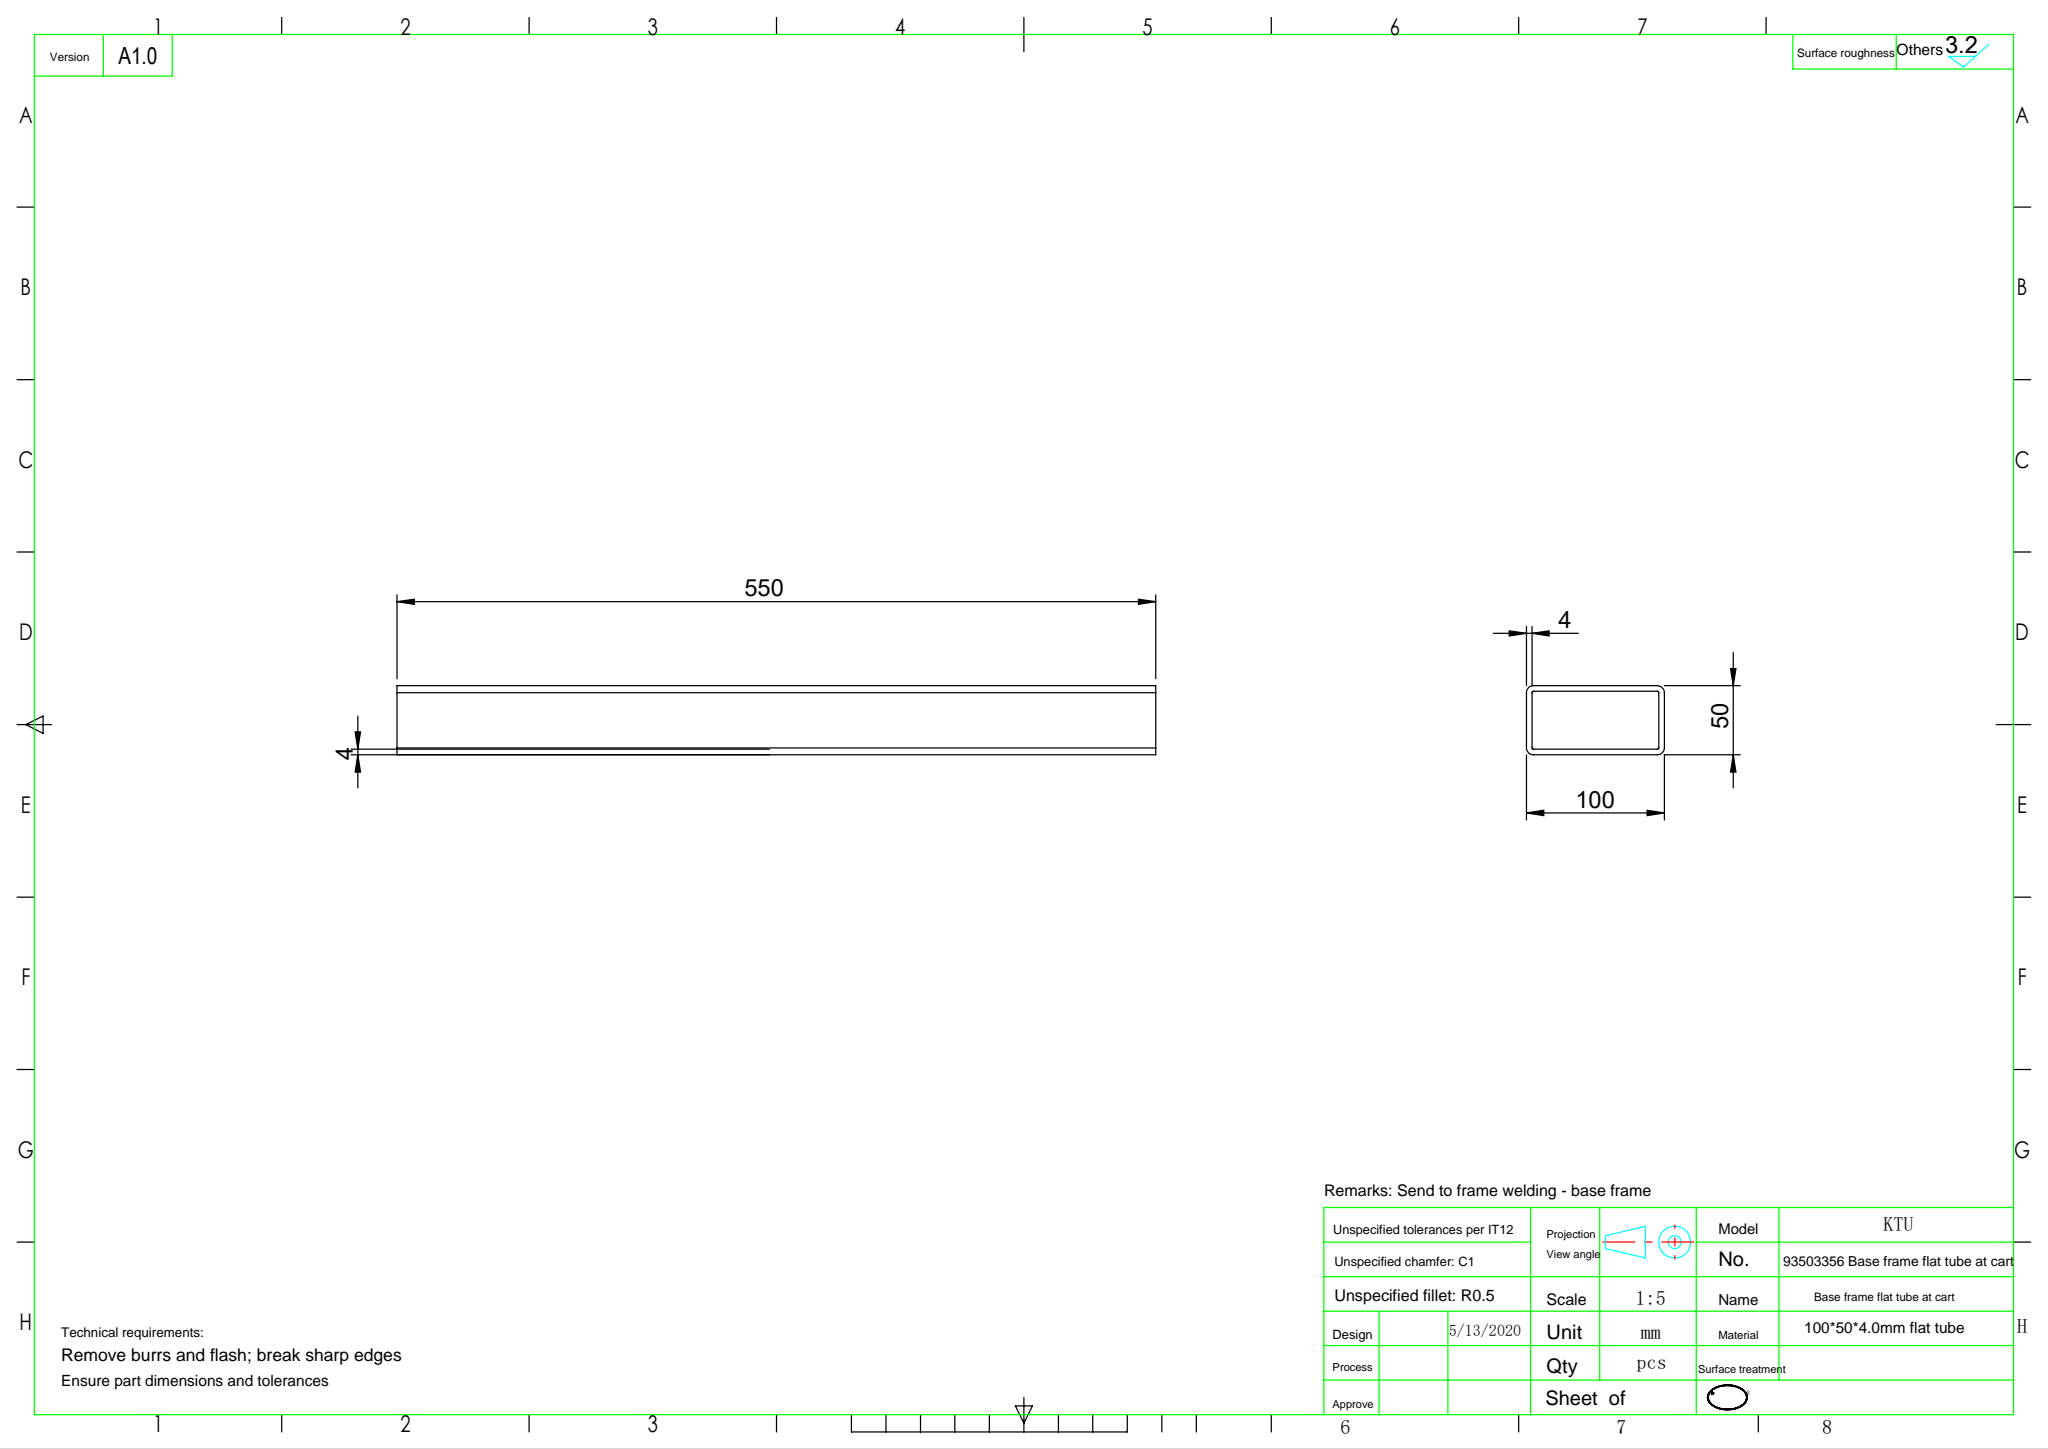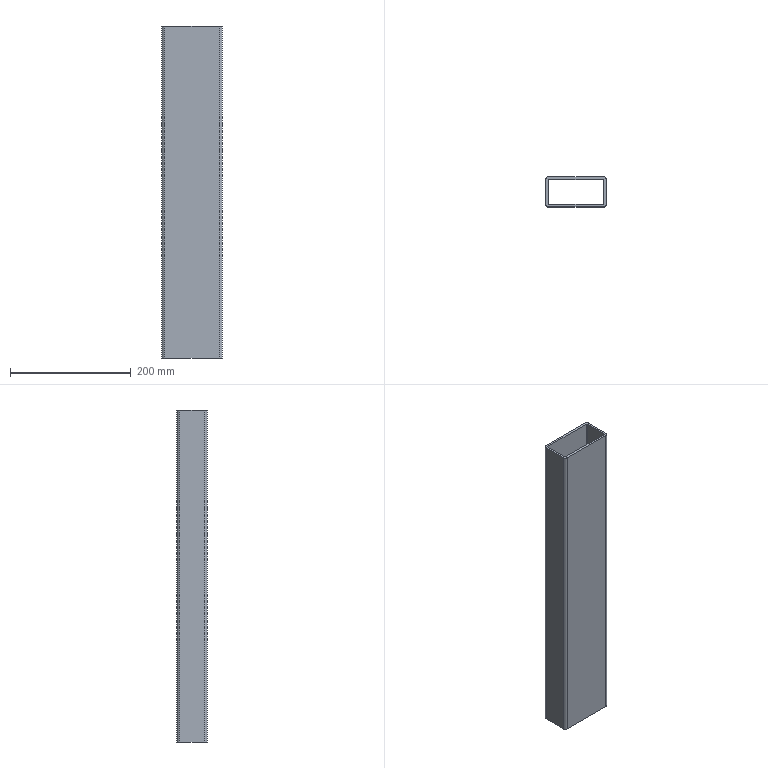Part | SolidWorks | features ExtruThin 1 | 1 solid | 18 faces | box 100 x 50 x 550 mm | volume 613469 mm3 | plane 10 | cylinder 8 | commonest cylinder face diameters 2 x4 10 x4
STEP:
#1=CARTESIAN_POINT('',(45.,-25.,275.));
#2=VERTEX_POINT('',#1);
#3=CARTESIAN_POINT('',(50.,-20.,275.));
#4=VERTEX_POINT('',#3);
#5=CARTESIAN_POINT('',(45.,-20.,275.));
#6=DIRECTION('',(0.,0.,1.));
#7=DIRECTION('',(1.,0.,0.));
#8=AXIS2_PLACEMENT_3D('',#5,#6,#7);
#9=CIRCLE('',#8,5.);
#10=EDGE_CURVE('',#2,#4,#9,.T.);
#11=ORIENTED_EDGE('',*,*,#10,.T.);
#12=CARTESIAN_POINT('',(50.,20.,275.));
#13=VERTEX_POINT('',#12);
#14=CARTESIAN_POINT('',(50.,20.,275.));
#15=DIRECTION('',(0.,1.,0.));
#16=VECTOR('',#15,1000.);
#17=LINE('',#14,#16);
#18=EDGE_CURVE('',#4,#13,#17,.T.);
#19=ORIENTED_EDGE('',*,*,#18,.T.);
#20=CARTESIAN_POINT('',(45.,25.,275.));
#21=VERTEX_POINT('',#20);
#22=CARTESIAN_POINT('',(45.,20.,275.));
#23=DIRECTION('',(0.,0.,1.));
#24=DIRECTION('',(-1.,0.,0.));
#25=AXIS2_PLACEMENT_3D('',#22,#23,#24);
#26=CIRCLE('',#25,5.);
#27=EDGE_CURVE('',#13,#21,#26,.T.);
#28=ORIENTED_EDGE('',*,*,#27,.T.);
#29=CARTESIAN_POINT('',(-45.,25.,275.));
#30=VERTEX_POINT('',#29);
#31=CARTESIAN_POINT('',(-45.,25.,275.));
#32=DIRECTION('',(-1.,0.,0.));
#33=VECTOR('',#32,1000.);
#34=LINE('',#31,#33);
#35=EDGE_CURVE('',#21,#30,#34,.T.);
#36=ORIENTED_EDGE('',*,*,#35,.T.);
#37=CARTESIAN_POINT('',(-50.,20.,275.));
#38=VERTEX_POINT('',#37);
#39=CARTESIAN_POINT('',(-45.,20.,275.));
#40=DIRECTION('',(0.,0.,1.));
#41=DIRECTION('',(1.,0.,0.));
#42=AXIS2_PLACEMENT_3D('',#39,#40,#41);
#43=CIRCLE('',#42,5.);
#44=EDGE_CURVE('',#30,#38,#43,.T.);
#45=ORIENTED_EDGE('',*,*,#44,.T.);
#46=CARTESIAN_POINT('',(-50.,-20.,275.));
#47=VERTEX_POINT('',#46);
#48=CARTESIAN_POINT('',(-50.,20.,275.));
#49=DIRECTION('',(0.,-1.,0.));
#50=VECTOR('',#49,1000.);
#51=LINE('',#48,#50);
#52=EDGE_CURVE('',#38,#47,#51,.T.);
#53=ORIENTED_EDGE('',*,*,#52,.T.);
#54=CARTESIAN_POINT('',(-45.,-25.,275.));
#55=VERTEX_POINT('',#54);
#56=CARTESIAN_POINT('',(-45.,-20.,275.));
#57=DIRECTION('',(0.,0.,1.));
#58=DIRECTION('',(1.,0.,0.));
#59=AXIS2_PLACEMENT_3D('',#56,#57,#58);
#60=CIRCLE('',#59,5.);
#61=EDGE_CURVE('',#47,#55,#60,.T.);
#62=ORIENTED_EDGE('',*,*,#61,.T.);
#63=CARTESIAN_POINT('',(-45.,-25.,275.));
#64=DIRECTION('',(1.,0.,0.));
#65=VECTOR('',#64,1000.);
#66=LINE('',#63,#65);
#67=EDGE_CURVE('',#55,#2,#66,.T.);
#68=ORIENTED_EDGE('',*,*,#67,.T.);
#69=EDGE_LOOP('',(#11,#19,#28,#36,#45,#53,#62,#68));
#70=FACE_OUTER_BOUND('',#69,.T.);
#71=CARTESIAN_POINT('',(46.,-20.,275.));
#72=VERTEX_POINT('',#71);
#73=CARTESIAN_POINT('',(46.,20.,275.));
#74=VERTEX_POINT('',#73);
#75=CARTESIAN_POINT('',(46.,20.,275.));
#76=DIRECTION('',(0.,1.,0.));
#77=VECTOR('',#76,1000.);
#78=LINE('',#75,#77);
#79=EDGE_CURVE('',#72,#74,#78,.T.);
#80=ORIENTED_EDGE('',*,*,#79,.F.);
#81=CARTESIAN_POINT('',(45.,-21.,275.));
#82=VERTEX_POINT('',#81);
#83=CARTESIAN_POINT('',(45.,-20.,275.));
#84=DIRECTION('',(0.,0.,1.));
#85=DIRECTION('',(1.,0.,0.));
#86=AXIS2_PLACEMENT_3D('',#83,#84,#85);
#87=CIRCLE('',#86,1.);
#88=EDGE_CURVE('',#82,#72,#87,.T.);
#89=ORIENTED_EDGE('',*,*,#88,.F.);
#90=CARTESIAN_POINT('',(-45.,-21.,275.));
#91=VERTEX_POINT('',#90);
#92=CARTESIAN_POINT('',(-45.,-21.,275.));
#93=DIRECTION('',(1.,0.,0.));
#94=VECTOR('',#93,1000.);
#95=LINE('',#92,#94);
#96=EDGE_CURVE('',#91,#82,#95,.T.);
#97=ORIENTED_EDGE('',*,*,#96,.F.);
#98=CARTESIAN_POINT('',(-46.,-20.,275.));
#99=VERTEX_POINT('',#98);
#100=CARTESIAN_POINT('',(-45.,-20.,275.));
#101=DIRECTION('',(0.,0.,1.));
#102=DIRECTION('',(1.,0.,0.));
#103=AXIS2_PLACEMENT_3D('',#100,#101,#102);
#104=CIRCLE('',#103,1.);
#105=EDGE_CURVE('',#99,#91,#104,.T.);
#106=ORIENTED_EDGE('',*,*,#105,.F.);
#107=CARTESIAN_POINT('',(-46.,20.,275.));
#108=VERTEX_POINT('',#107);
#109=CARTESIAN_POINT('',(-46.,20.,275.));
#110=DIRECTION('',(0.,-1.,0.));
#111=VECTOR('',#110,1000.);
#112=LINE('',#109,#111);
#113=EDGE_CURVE('',#108,#99,#112,.T.);
#114=ORIENTED_EDGE('',*,*,#113,.F.);
#115=CARTESIAN_POINT('',(-45.,21.,275.));
#116=VERTEX_POINT('',#115);
#117=CARTESIAN_POINT('',(-45.,20.,275.));
#118=DIRECTION('',(0.,0.,1.));
#119=DIRECTION('',(1.,0.,0.));
#120=AXIS2_PLACEMENT_3D('',#117,#118,#119);
#121=CIRCLE('',#120,1.);
#122=EDGE_CURVE('',#116,#108,#121,.T.);
#123=ORIENTED_EDGE('',*,*,#122,.F.);
#124=CARTESIAN_POINT('',(45.,21.,275.));
#125=VERTEX_POINT('',#124);
#126=CARTESIAN_POINT('',(-45.,21.,275.));
#127=DIRECTION('',(-1.,0.,0.));
#128=VECTOR('',#127,1000.);
#129=LINE('',#126,#128);
#130=EDGE_CURVE('',#125,#116,#129,.T.);
#131=ORIENTED_EDGE('',*,*,#130,.F.);
#132=CARTESIAN_POINT('',(45.,20.,275.));
#133=DIRECTION('',(0.,0.,1.));
#134=DIRECTION('',(1.,0.,0.));
#135=AXIS2_PLACEMENT_3D('',#132,#133,#134);
#136=CIRCLE('',#135,1.);
#137=EDGE_CURVE('',#74,#125,#136,.T.);
#138=ORIENTED_EDGE('',*,*,#137,.F.);
#139=EDGE_LOOP('',(#80,#89,#97,#106,#114,#123,#131,#138));
#140=FACE_BOUND('',#139,.T.);
#141=CARTESIAN_POINT('',(45.,-20.,275.));
#142=DIRECTION('',(0.,0.,1.));
#143=DIRECTION('',(1.,0.,0.));
#144=AXIS2_PLACEMENT_3D('',#141,#142,#143);
#145=PLANE('',#144);
#146=ADVANCED_FACE('',(#70,#140),#145,.T.);
#147=CARTESIAN_POINT('',(45.,-25.,-275.));
#148=VERTEX_POINT('',#147);
#149=CARTESIAN_POINT('',(50.,-20.,-275.));
#150=VERTEX_POINT('',#149);
#151=CARTESIAN_POINT('',(45.,-20.,-275.));
#152=DIRECTION('',(0.,0.,1.));
#153=DIRECTION('',(1.,0.,0.));
#154=AXIS2_PLACEMENT_3D('',#151,#152,#153);
#155=CIRCLE('',#154,5.);
#156=EDGE_CURVE('',#148,#150,#155,.T.);
#157=ORIENTED_EDGE('',*,*,#156,.F.);
#158=CARTESIAN_POINT('',(-45.,-25.,-275.));
#159=VERTEX_POINT('',#158);
#160=CARTESIAN_POINT('',(-45.,-25.,-275.));
#161=DIRECTION('',(1.,0.,0.));
#162=VECTOR('',#161,1000.);
#163=LINE('',#160,#162);
#164=EDGE_CURVE('',#159,#148,#163,.T.);
#165=ORIENTED_EDGE('',*,*,#164,.F.);
#166=CARTESIAN_POINT('',(-50.,-20.,-275.));
#167=VERTEX_POINT('',#166);
#168=CARTESIAN_POINT('',(-45.,-20.,-275.));
#169=DIRECTION('',(0.,0.,1.));
#170=DIRECTION('',(1.,0.,0.));
#171=AXIS2_PLACEMENT_3D('',#168,#169,#170);
#172=CIRCLE('',#171,5.);
#173=EDGE_CURVE('',#167,#159,#172,.T.);
#174=ORIENTED_EDGE('',*,*,#173,.F.);
#175=CARTESIAN_POINT('',(-50.,20.,-275.));
#176=VERTEX_POINT('',#175);
#177=CARTESIAN_POINT('',(-50.,20.,-275.));
#178=DIRECTION('',(0.,-1.,0.));
#179=VECTOR('',#178,1000.);
#180=LINE('',#177,#179);
#181=EDGE_CURVE('',#176,#167,#180,.T.);
#182=ORIENTED_EDGE('',*,*,#181,.F.);
#183=CARTESIAN_POINT('',(-45.,25.,-275.));
#184=VERTEX_POINT('',#183);
#185=CARTESIAN_POINT('',(-45.,20.,-275.));
#186=DIRECTION('',(0.,0.,1.));
#187=DIRECTION('',(1.,0.,0.));
#188=AXIS2_PLACEMENT_3D('',#185,#186,#187);
#189=CIRCLE('',#188,5.);
#190=EDGE_CURVE('',#184,#176,#189,.T.);
#191=ORIENTED_EDGE('',*,*,#190,.F.);
#192=CARTESIAN_POINT('',(45.,25.,-275.));
#193=VERTEX_POINT('',#192);
#194=CARTESIAN_POINT('',(-45.,25.,-275.));
#195=DIRECTION('',(-1.,0.,0.));
#196=VECTOR('',#195,1000.);
#197=LINE('',#194,#196);
#198=EDGE_CURVE('',#193,#184,#197,.T.);
#199=ORIENTED_EDGE('',*,*,#198,.F.);
#200=CARTESIAN_POINT('',(50.,20.,-275.));
#201=VERTEX_POINT('',#200);
#202=CARTESIAN_POINT('',(45.,20.,-275.));
#203=DIRECTION('',(0.,0.,1.));
#204=DIRECTION('',(-1.,0.,0.));
#205=AXIS2_PLACEMENT_3D('',#202,#203,#204);
#206=CIRCLE('',#205,5.);
#207=EDGE_CURVE('',#201,#193,#206,.T.);
#208=ORIENTED_EDGE('',*,*,#207,.F.);
#209=CARTESIAN_POINT('',(50.,20.,-275.));
#210=DIRECTION('',(0.,1.,0.));
#211=VECTOR('',#210,1000.);
#212=LINE('',#209,#211);
#213=EDGE_CURVE('',#150,#201,#212,.T.);
#214=ORIENTED_EDGE('',*,*,#213,.F.);
#215=EDGE_LOOP('',(#157,#165,#174,#182,#191,#199,#208,#214));
#216=FACE_OUTER_BOUND('',#215,.T.);
#217=CARTESIAN_POINT('',(45.,-21.,-275.));
#218=VERTEX_POINT('',#217);
#219=CARTESIAN_POINT('',(46.,-20.,-275.));
#220=VERTEX_POINT('',#219);
#221=CARTESIAN_POINT('',(45.,-20.,-275.));
#222=DIRECTION('',(0.,0.,1.));
#223=DIRECTION('',(1.,0.,0.));
#224=AXIS2_PLACEMENT_3D('',#221,#222,#223);
#225=CIRCLE('',#224,1.);
#226=EDGE_CURVE('',#218,#220,#225,.T.);
#227=ORIENTED_EDGE('',*,*,#226,.T.);
#228=CARTESIAN_POINT('',(46.,20.,-275.));
#229=VERTEX_POINT('',#228);
#230=CARTESIAN_POINT('',(46.,20.,-275.));
#231=DIRECTION('',(0.,1.,0.));
#232=VECTOR('',#231,1000.);
#233=LINE('',#230,#232);
#234=EDGE_CURVE('',#220,#229,#233,.T.);
#235=ORIENTED_EDGE('',*,*,#234,.T.);
#236=CARTESIAN_POINT('',(45.,21.,-275.));
#237=VERTEX_POINT('',#236);
#238=CARTESIAN_POINT('',(45.,20.,-275.));
#239=DIRECTION('',(0.,0.,1.));
#240=DIRECTION('',(1.,0.,0.));
#241=AXIS2_PLACEMENT_3D('',#238,#239,#240);
#242=CIRCLE('',#241,1.);
#243=EDGE_CURVE('',#229,#237,#242,.T.);
#244=ORIENTED_EDGE('',*,*,#243,.T.);
#245=CARTESIAN_POINT('',(-45.,21.,-275.));
#246=VERTEX_POINT('',#245);
#247=CARTESIAN_POINT('',(-45.,21.,-275.));
#248=DIRECTION('',(-1.,0.,0.));
#249=VECTOR('',#248,1000.);
#250=LINE('',#247,#249);
#251=EDGE_CURVE('',#237,#246,#250,.T.);
#252=ORIENTED_EDGE('',*,*,#251,.T.);
#253=CARTESIAN_POINT('',(-46.,20.,-275.));
#254=VERTEX_POINT('',#253);
#255=CARTESIAN_POINT('',(-45.,20.,-275.));
#256=DIRECTION('',(0.,0.,1.));
#257=DIRECTION('',(1.,0.,0.));
#258=AXIS2_PLACEMENT_3D('',#255,#256,#257);
#259=CIRCLE('',#258,1.);
#260=EDGE_CURVE('',#246,#254,#259,.T.);
#261=ORIENTED_EDGE('',*,*,#260,.T.);
#262=CARTESIAN_POINT('',(-46.,-20.,-275.));
#263=VERTEX_POINT('',#262);
#264=CARTESIAN_POINT('',(-46.,20.,-275.));
#265=DIRECTION('',(0.,-1.,0.));
#266=VECTOR('',#265,1000.);
#267=LINE('',#264,#266);
#268=EDGE_CURVE('',#254,#263,#267,.T.);
#269=ORIENTED_EDGE('',*,*,#268,.T.);
#270=CARTESIAN_POINT('',(-45.,-21.,-275.));
#271=VERTEX_POINT('',#270);
#272=CARTESIAN_POINT('',(-45.,-20.,-275.));
#273=DIRECTION('',(0.,0.,1.));
#274=DIRECTION('',(1.,0.,0.));
#275=AXIS2_PLACEMENT_3D('',#272,#273,#274);
#276=CIRCLE('',#275,1.);
#277=EDGE_CURVE('',#263,#271,#276,.T.);
#278=ORIENTED_EDGE('',*,*,#277,.T.);
#279=CARTESIAN_POINT('',(-45.,-21.,-275.));
#280=DIRECTION('',(1.,0.,0.));
#281=VECTOR('',#280,1000.);
#282=LINE('',#279,#281);
#283=EDGE_CURVE('',#271,#218,#282,.T.);
#284=ORIENTED_EDGE('',*,*,#283,.T.);
#285=EDGE_LOOP('',(#227,#235,#244,#252,#261,#269,#278,#284));
#286=FACE_BOUND('',#285,.T.);
#287=CARTESIAN_POINT('',(45.,-20.,-275.));
#288=DIRECTION('',(0.,0.,1.));
#289=DIRECTION('',(1.,0.,0.));
#290=AXIS2_PLACEMENT_3D('',#287,#288,#289);
#291=PLANE('',#290);
#292=ADVANCED_FACE('',(#216,#286),#291,.F.);
#293=ORIENTED_EDGE('',*,*,#156,.T.);
#294=CARTESIAN_POINT('',(50.,-20.,275.));
#295=DIRECTION('',(0.,0.,-1.));
#296=VECTOR('',#295,1000.);
#297=LINE('',#294,#296);
#298=EDGE_CURVE('',#4,#150,#297,.T.);
#299=ORIENTED_EDGE('',*,*,#298,.F.);
#300=ORIENTED_EDGE('',*,*,#10,.F.);
#301=CARTESIAN_POINT('',(45.,-25.,275.));
#302=DIRECTION('',(0.,0.,-1.));
#303=VECTOR('',#302,1000.);
#304=LINE('',#301,#303);
#305=EDGE_CURVE('',#2,#148,#304,.T.);
#306=ORIENTED_EDGE('',*,*,#305,.T.);
#307=EDGE_LOOP('',(#293,#299,#300,#306));
#308=FACE_OUTER_BOUND('',#307,.T.);
#309=CARTESIAN_POINT('',(45.,-20.,275.));
#310=DIRECTION('',(0.,0.,-1.));
#311=DIRECTION('',(-1.,0.,0.));
#312=AXIS2_PLACEMENT_3D('',#309,#310,#311);
#313=CYLINDRICAL_SURFACE('',#312,5.);
#314=ADVANCED_FACE('',(#308),#313,.T.);
#315=ORIENTED_EDGE('',*,*,#213,.T.);
#316=CARTESIAN_POINT('',(50.,20.,275.));
#317=DIRECTION('',(0.,0.,-1.));
#318=VECTOR('',#317,1000.);
#319=LINE('',#316,#318);
#320=EDGE_CURVE('',#13,#201,#319,.T.);
#321=ORIENTED_EDGE('',*,*,#320,.F.);
#322=ORIENTED_EDGE('',*,*,#18,.F.);
#323=ORIENTED_EDGE('',*,*,#298,.T.);
#324=EDGE_LOOP('',(#315,#321,#322,#323));
#325=FACE_OUTER_BOUND('',#324,.T.);
#326=CARTESIAN_POINT('',(50.,20.,275.));
#327=DIRECTION('',(-1.,0.,0.));
#328=DIRECTION('',(0.,-1.,0.));
#329=AXIS2_PLACEMENT_3D('',#326,#327,#328);
#330=PLANE('',#329);
#331=ADVANCED_FACE('',(#325),#330,.F.);
#332=ORIENTED_EDGE('',*,*,#207,.T.);
#333=CARTESIAN_POINT('',(45.,25.,275.));
#334=DIRECTION('',(0.,0.,-1.));
#335=VECTOR('',#334,1000.);
#336=LINE('',#333,#335);
#337=EDGE_CURVE('',#21,#193,#336,.T.);
#338=ORIENTED_EDGE('',*,*,#337,.F.);
#339=ORIENTED_EDGE('',*,*,#27,.F.);
#340=ORIENTED_EDGE('',*,*,#320,.T.);
#341=EDGE_LOOP('',(#332,#338,#339,#340));
#342=FACE_OUTER_BOUND('',#341,.T.);
#343=CARTESIAN_POINT('',(45.,20.,275.));
#344=DIRECTION('',(0.,0.,-1.));
#345=DIRECTION('',(-1.,0.,0.));
#346=AXIS2_PLACEMENT_3D('',#343,#344,#345);
#347=CYLINDRICAL_SURFACE('',#346,5.);
#348=ADVANCED_FACE('',(#342),#347,.T.);
#349=ORIENTED_EDGE('',*,*,#198,.T.);
#350=CARTESIAN_POINT('',(-45.,25.,275.));
#351=DIRECTION('',(0.,0.,-1.));
#352=VECTOR('',#351,1000.);
#353=LINE('',#350,#352);
#354=EDGE_CURVE('',#30,#184,#353,.T.);
#355=ORIENTED_EDGE('',*,*,#354,.F.);
#356=ORIENTED_EDGE('',*,*,#35,.F.);
#357=ORIENTED_EDGE('',*,*,#337,.T.);
#358=EDGE_LOOP('',(#349,#355,#356,#357));
#359=FACE_OUTER_BOUND('',#358,.T.);
#360=CARTESIAN_POINT('',(-45.,25.,275.));
#361=DIRECTION('',(0.,-1.,0.));
#362=DIRECTION('',(0.,0.,-1.));
#363=AXIS2_PLACEMENT_3D('',#360,#361,#362);
#364=PLANE('',#363);
#365=ADVANCED_FACE('',(#359),#364,.F.);
#366=ORIENTED_EDGE('',*,*,#190,.T.);
#367=CARTESIAN_POINT('',(-50.,20.,275.));
#368=DIRECTION('',(0.,0.,-1.));
#369=VECTOR('',#368,1000.);
#370=LINE('',#367,#369);
#371=EDGE_CURVE('',#38,#176,#370,.T.);
#372=ORIENTED_EDGE('',*,*,#371,.F.);
#373=ORIENTED_EDGE('',*,*,#44,.F.);
#374=ORIENTED_EDGE('',*,*,#354,.T.);
#375=EDGE_LOOP('',(#366,#372,#373,#374));
#376=FACE_OUTER_BOUND('',#375,.T.);
#377=CARTESIAN_POINT('',(-45.,20.,275.));
#378=DIRECTION('',(0.,0.,-1.));
#379=DIRECTION('',(-1.,0.,0.));
#380=AXIS2_PLACEMENT_3D('',#377,#378,#379);
#381=CYLINDRICAL_SURFACE('',#380,5.);
#382=ADVANCED_FACE('',(#376),#381,.T.);
#383=ORIENTED_EDGE('',*,*,#181,.T.);
#384=CARTESIAN_POINT('',(-50.,-20.,275.));
#385=DIRECTION('',(0.,0.,-1.));
#386=VECTOR('',#385,1000.);
#387=LINE('',#384,#386);
#388=EDGE_CURVE('',#47,#167,#387,.T.);
#389=ORIENTED_EDGE('',*,*,#388,.F.);
#390=ORIENTED_EDGE('',*,*,#52,.F.);
#391=ORIENTED_EDGE('',*,*,#371,.T.);
#392=EDGE_LOOP('',(#383,#389,#390,#391));
#393=FACE_OUTER_BOUND('',#392,.T.);
#394=CARTESIAN_POINT('',(-50.,20.,275.));
#395=DIRECTION('',(1.,0.,0.));
#396=DIRECTION('',(0.,0.,-1.));
#397=AXIS2_PLACEMENT_3D('',#394,#395,#396);
#398=PLANE('',#397);
#399=ADVANCED_FACE('',(#393),#398,.F.);
#400=ORIENTED_EDGE('',*,*,#173,.T.);
#401=CARTESIAN_POINT('',(-45.,-25.,275.));
#402=DIRECTION('',(0.,0.,-1.));
#403=VECTOR('',#402,1000.);
#404=LINE('',#401,#403);
#405=EDGE_CURVE('',#55,#159,#404,.T.);
#406=ORIENTED_EDGE('',*,*,#405,.F.);
#407=ORIENTED_EDGE('',*,*,#61,.F.);
#408=ORIENTED_EDGE('',*,*,#388,.T.);
#409=EDGE_LOOP('',(#400,#406,#407,#408));
#410=FACE_OUTER_BOUND('',#409,.T.);
#411=CARTESIAN_POINT('',(-45.,-20.,275.));
#412=DIRECTION('',(0.,0.,-1.));
#413=DIRECTION('',(-1.,0.,0.));
#414=AXIS2_PLACEMENT_3D('',#411,#412,#413);
#415=CYLINDRICAL_SURFACE('',#414,5.);
#416=ADVANCED_FACE('',(#410),#415,.T.);
#417=ORIENTED_EDGE('',*,*,#164,.T.);
#418=ORIENTED_EDGE('',*,*,#305,.F.);
#419=ORIENTED_EDGE('',*,*,#67,.F.);
#420=ORIENTED_EDGE('',*,*,#405,.T.);
#421=EDGE_LOOP('',(#417,#418,#419,#420));
#422=FACE_OUTER_BOUND('',#421,.T.);
#423=CARTESIAN_POINT('',(-45.,-25.,275.));
#424=DIRECTION('',(0.,1.,0.));
#425=DIRECTION('',(0.,0.,1.));
#426=AXIS2_PLACEMENT_3D('',#423,#424,#425);
#427=PLANE('',#426);
#428=ADVANCED_FACE('',(#422),#427,.F.);
#429=ORIENTED_EDGE('',*,*,#226,.F.);
#430=CARTESIAN_POINT('',(45.,-21.,275.));
#431=DIRECTION('',(0.,0.,-1.));
#432=VECTOR('',#431,1000.);
#433=LINE('',#430,#432);
#434=EDGE_CURVE('',#82,#218,#433,.T.);
#435=ORIENTED_EDGE('',*,*,#434,.F.);
#436=ORIENTED_EDGE('',*,*,#88,.T.);
#437=CARTESIAN_POINT('',(46.,-20.,275.));
#438=DIRECTION('',(0.,0.,-1.));
#439=VECTOR('',#438,1000.);
#440=LINE('',#437,#439);
#441=EDGE_CURVE('',#72,#220,#440,.T.);
#442=ORIENTED_EDGE('',*,*,#441,.T.);
#443=EDGE_LOOP('',(#429,#435,#436,#442));
#444=FACE_OUTER_BOUND('',#443,.T.);
#445=CARTESIAN_POINT('',(45.,-20.,275.));
#446=DIRECTION('',(0.,0.,-1.));
#447=DIRECTION('',(-1.,0.,0.));
#448=AXIS2_PLACEMENT_3D('',#445,#446,#447);
#449=CYLINDRICAL_SURFACE('',#448,1.);
#450=ADVANCED_FACE('',(#444),#449,.F.);
#451=ORIENTED_EDGE('',*,*,#234,.F.);
#452=ORIENTED_EDGE('',*,*,#441,.F.);
#453=ORIENTED_EDGE('',*,*,#79,.T.);
#454=CARTESIAN_POINT('',(46.,20.,275.));
#455=DIRECTION('',(0.,0.,-1.));
#456=VECTOR('',#455,1000.);
#457=LINE('',#454,#456);
#458=EDGE_CURVE('',#74,#229,#457,.T.);
#459=ORIENTED_EDGE('',*,*,#458,.T.);
#460=EDGE_LOOP('',(#451,#452,#453,#459));
#461=FACE_OUTER_BOUND('',#460,.T.);
#462=CARTESIAN_POINT('',(46.,20.,275.));
#463=DIRECTION('',(-1.,0.,0.));
#464=DIRECTION('',(0.,-1.,0.));
#465=AXIS2_PLACEMENT_3D('',#462,#463,#464);
#466=PLANE('',#465);
#467=ADVANCED_FACE('',(#461),#466,.T.);
#468=ORIENTED_EDGE('',*,*,#243,.F.);
#469=ORIENTED_EDGE('',*,*,#458,.F.);
#470=ORIENTED_EDGE('',*,*,#137,.T.);
#471=CARTESIAN_POINT('',(45.,21.,275.));
#472=DIRECTION('',(0.,0.,-1.));
#473=VECTOR('',#472,1000.);
#474=LINE('',#471,#473);
#475=EDGE_CURVE('',#125,#237,#474,.T.);
#476=ORIENTED_EDGE('',*,*,#475,.T.);
#477=EDGE_LOOP('',(#468,#469,#470,#476));
#478=FACE_OUTER_BOUND('',#477,.T.);
#479=CARTESIAN_POINT('',(45.,20.,275.));
#480=DIRECTION('',(0.,0.,-1.));
#481=DIRECTION('',(-1.,0.,0.));
#482=AXIS2_PLACEMENT_3D('',#479,#480,#481);
#483=CYLINDRICAL_SURFACE('',#482,1.);
#484=ADVANCED_FACE('',(#478),#483,.F.);
#485=ORIENTED_EDGE('',*,*,#251,.F.);
#486=ORIENTED_EDGE('',*,*,#475,.F.);
#487=ORIENTED_EDGE('',*,*,#130,.T.);
#488=CARTESIAN_POINT('',(-45.,21.,275.));
#489=DIRECTION('',(0.,0.,-1.));
#490=VECTOR('',#489,1000.);
#491=LINE('',#488,#490);
#492=EDGE_CURVE('',#116,#246,#491,.T.);
#493=ORIENTED_EDGE('',*,*,#492,.T.);
#494=EDGE_LOOP('',(#485,#486,#487,#493));
#495=FACE_OUTER_BOUND('',#494,.T.);
#496=CARTESIAN_POINT('',(-45.,21.,275.));
#497=DIRECTION('',(0.,-1.,0.));
#498=DIRECTION('',(0.,0.,-1.));
#499=AXIS2_PLACEMENT_3D('',#496,#497,#498);
#500=PLANE('',#499);
#501=ADVANCED_FACE('',(#495),#500,.T.);
#502=ORIENTED_EDGE('',*,*,#260,.F.);
#503=ORIENTED_EDGE('',*,*,#492,.F.);
#504=ORIENTED_EDGE('',*,*,#122,.T.);
#505=CARTESIAN_POINT('',(-46.,20.,275.));
#506=DIRECTION('',(0.,0.,-1.));
#507=VECTOR('',#506,1000.);
#508=LINE('',#505,#507);
#509=EDGE_CURVE('',#108,#254,#508,.T.);
#510=ORIENTED_EDGE('',*,*,#509,.T.);
#511=EDGE_LOOP('',(#502,#503,#504,#510));
#512=FACE_OUTER_BOUND('',#511,.T.);
#513=CARTESIAN_POINT('',(-45.,20.,275.));
#514=DIRECTION('',(0.,0.,-1.));
#515=DIRECTION('',(-1.,0.,0.));
#516=AXIS2_PLACEMENT_3D('',#513,#514,#515);
#517=CYLINDRICAL_SURFACE('',#516,1.);
#518=ADVANCED_FACE('',(#512),#517,.F.);
#519=ORIENTED_EDGE('',*,*,#268,.F.);
#520=ORIENTED_EDGE('',*,*,#509,.F.);
#521=ORIENTED_EDGE('',*,*,#113,.T.);
#522=CARTESIAN_POINT('',(-46.,-20.,275.));
#523=DIRECTION('',(0.,0.,-1.));
#524=VECTOR('',#523,1000.);
#525=LINE('',#522,#524);
#526=EDGE_CURVE('',#99,#263,#525,.T.);
#527=ORIENTED_EDGE('',*,*,#526,.T.);
#528=EDGE_LOOP('',(#519,#520,#521,#527));
#529=FACE_OUTER_BOUND('',#528,.T.);
#530=CARTESIAN_POINT('',(-46.,20.,275.));
#531=DIRECTION('',(1.,0.,0.));
#532=DIRECTION('',(0.,0.,-1.));
#533=AXIS2_PLACEMENT_3D('',#530,#531,#532);
#534=PLANE('',#533);
#535=ADVANCED_FACE('',(#529),#534,.T.);
#536=ORIENTED_EDGE('',*,*,#277,.F.);
#537=ORIENTED_EDGE('',*,*,#526,.F.);
#538=ORIENTED_EDGE('',*,*,#105,.T.);
#539=CARTESIAN_POINT('',(-45.,-21.,275.));
#540=DIRECTION('',(0.,0.,-1.));
#541=VECTOR('',#540,1000.);
#542=LINE('',#539,#541);
#543=EDGE_CURVE('',#91,#271,#542,.T.);
#544=ORIENTED_EDGE('',*,*,#543,.T.);
#545=EDGE_LOOP('',(#536,#537,#538,#544));
#546=FACE_OUTER_BOUND('',#545,.T.);
#547=CARTESIAN_POINT('',(-45.,-20.,275.));
#548=DIRECTION('',(0.,0.,-1.));
#549=DIRECTION('',(-1.,0.,0.));
#550=AXIS2_PLACEMENT_3D('',#547,#548,#549);
#551=CYLINDRICAL_SURFACE('',#550,1.);
#552=ADVANCED_FACE('',(#546),#551,.F.);
#553=ORIENTED_EDGE('',*,*,#283,.F.);
#554=ORIENTED_EDGE('',*,*,#543,.F.);
#555=ORIENTED_EDGE('',*,*,#96,.T.);
#556=ORIENTED_EDGE('',*,*,#434,.T.);
#557=EDGE_LOOP('',(#553,#554,#555,#556));
#558=FACE_OUTER_BOUND('',#557,.T.);
#559=CARTESIAN_POINT('',(-45.,-21.,275.));
#560=DIRECTION('',(0.,1.,0.));
#561=DIRECTION('',(0.,0.,1.));
#562=AXIS2_PLACEMENT_3D('',#559,#560,#561);
#563=PLANE('',#562);
#564=ADVANCED_FACE('',(#558),#563,.T.);
#565=CLOSED_SHELL('',(#146,#292,#314,#331,#348,#365,#382,#399,#416,#428,#450,#467,#484,#501,#518,#535,#552,#564));
#566=MANIFOLD_SOLID_BREP('',#565);
#567=CARTESIAN_POINT('',(0.,0.,0.));
#568=DIRECTION('',(0.,0.,1.));
#569=DIRECTION('',(1.,0.,0.));
#570=AXIS2_PLACEMENT_3D('',#567,#568,#569);
#571=(LENGTH_UNIT()NAMED_UNIT(*)SI_UNIT(.MILLI.,.METRE.));
#572=UNCERTAINTY_MEASURE_WITH_UNIT(LENGTH_MEASURE(0.00001),#571,'','');
#573=(NAMED_UNIT(*)PLANE_ANGLE_UNIT()SI_UNIT($,.RADIAN.));
#574=(NAMED_UNIT(*)SI_UNIT($,.STERADIAN.)SOLID_ANGLE_UNIT());
#575=(GEOMETRIC_REPRESENTATION_CONTEXT(3)GLOBAL_UNCERTAINTY_ASSIGNED_CONTEXT((#572))GLOBAL_UNIT_ASSIGNED_CONTEXT((#571,#573,#574))REPRESENTATION_CONTEXT('',''));
#576=ADVANCED_BREP_SHAPE_REPRESENTATION('',(#566,#570),#575);